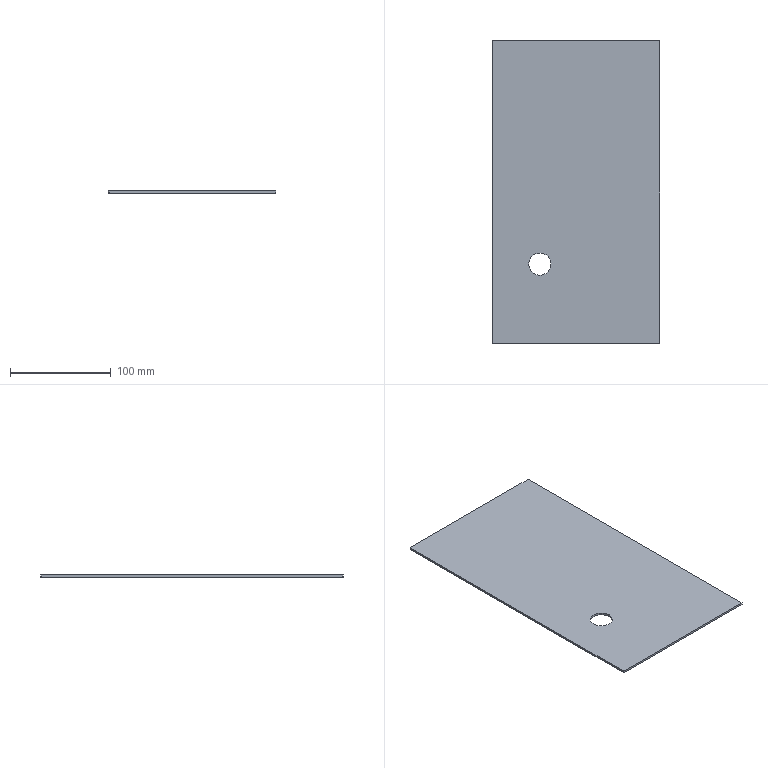Part | STEP file | Oil Filler Tank Closing Plate | 1 solid | 10 faces | box 166.5 x 301 x 2 mm | volume 99472 mm3 | plane 6 | cylinder 4 | commonest cylinder face diameters 1.5 x2 22 x2
STEP:
#1=CARTESIAN_POINT('',(-110.219,-71.7,-2.));
#2=VERTEX_POINT('',#1);
#3=CARTESIAN_POINT('',(-132.219,-71.7,-2.));
#4=VERTEX_POINT('',#3);
#5=CARTESIAN_POINT('',(-121.219,-71.7,-2.));
#6=DIRECTION('',(0.,0.,-1.));
#7=DIRECTION('',(1.,0.,0.));
#8=AXIS2_PLACEMENT_3D('',#5,#6,#7);
#9=CIRCLE('',#8,11.);
#10=EDGE_CURVE('',#2,#4,#9,.T.);
#11=ORIENTED_EDGE('',*,*,#10,.T.);
#12=CARTESIAN_POINT('',(-132.219,-71.7,0.));
#13=VERTEX_POINT('',#12);
#14=CARTESIAN_POINT('',(-132.219,-71.7,-10.));
#15=DIRECTION('',(0.,0.,1.));
#16=VECTOR('',#15,1000.);
#17=LINE('',#14,#16);
#18=EDGE_CURVE('',#4,#13,#17,.T.);
#19=ORIENTED_EDGE('',*,*,#18,.T.);
#20=CARTESIAN_POINT('',(-110.219,-71.7,0.));
#21=VERTEX_POINT('',#20);
#22=CARTESIAN_POINT('',(-121.219,-71.7,0.));
#23=DIRECTION('',(0.,0.,-1.));
#24=DIRECTION('',(1.,0.,0.));
#25=AXIS2_PLACEMENT_3D('',#22,#23,#24);
#26=CIRCLE('',#25,11.);
#27=EDGE_CURVE('',#21,#13,#26,.T.);
#28=ORIENTED_EDGE('',*,*,#27,.F.);
#29=CARTESIAN_POINT('',(-110.219,-71.7,-10.));
#30=DIRECTION('',(0.,0.,1.));
#31=VECTOR('',#30,1000.);
#32=LINE('',#29,#31);
#33=EDGE_CURVE('',#2,#21,#32,.T.);
#34=ORIENTED_EDGE('',*,*,#33,.F.);
#35=EDGE_LOOP('',(#11,#19,#28,#34));
#36=FACE_OUTER_BOUND('',#35,.T.);
#37=CARTESIAN_POINT('',(-121.219,-71.7,-10.));
#38=DIRECTION('',(0.,0.,1.));
#39=DIRECTION('',(1.,0.,0.));
#40=AXIS2_PLACEMENT_3D('',#37,#38,#39);
#41=CYLINDRICAL_SURFACE('',#40,11.);
#42=ADVANCED_FACE('',(#36),#41,.F.);
#43=CARTESIAN_POINT('',(-168.5,-149.75,-2.));
#44=VERTEX_POINT('',#43);
#45=CARTESIAN_POINT('',(-167.75,-150.5,-2.));
#46=VERTEX_POINT('',#45);
#47=CARTESIAN_POINT('',(-167.75,-149.75,-2.));
#48=DIRECTION('',(0.,0.,1.));
#49=DIRECTION('',(1.,0.,0.));
#50=AXIS2_PLACEMENT_3D('',#47,#48,#49);
#51=CIRCLE('',#50,0.75);
#52=EDGE_CURVE('',#44,#46,#51,.T.);
#53=ORIENTED_EDGE('',*,*,#52,.F.);
#54=CARTESIAN_POINT('',(-168.5,149.75,-2.));
#55=VERTEX_POINT('',#54);
#56=CARTESIAN_POINT('',(-168.5,0.,-2.));
#57=DIRECTION('',(0.,-1.,0.));
#58=VECTOR('',#57,1000.);
#59=LINE('',#56,#58);
#60=EDGE_CURVE('',#55,#44,#59,.T.);
#61=ORIENTED_EDGE('',*,*,#60,.F.);
#62=CARTESIAN_POINT('',(-167.75,150.5,-2.));
#63=VERTEX_POINT('',#62);
#64=CARTESIAN_POINT('',(-167.75,149.75,-2.));
#65=DIRECTION('',(0.,0.,1.));
#66=DIRECTION('',(1.,0.,0.));
#67=AXIS2_PLACEMENT_3D('',#64,#65,#66);
#68=CIRCLE('',#67,0.75);
#69=EDGE_CURVE('',#63,#55,#68,.T.);
#70=ORIENTED_EDGE('',*,*,#69,.F.);
#71=CARTESIAN_POINT('',(-2.,150.5,-2.));
#72=VERTEX_POINT('',#71);
#73=CARTESIAN_POINT('',(0.,150.5,-2.));
#74=DIRECTION('',(-1.,0.,0.));
#75=VECTOR('',#74,1000.);
#76=LINE('',#73,#75);
#77=EDGE_CURVE('',#72,#63,#76,.T.);
#78=ORIENTED_EDGE('',*,*,#77,.F.);
#79=CARTESIAN_POINT('',(-2.,-150.5,-2.));
#80=VERTEX_POINT('',#79);
#81=CARTESIAN_POINT('',(-2.,0.,-2.));
#82=DIRECTION('',(0.,1.,0.));
#83=VECTOR('',#82,1000.);
#84=LINE('',#81,#83);
#85=EDGE_CURVE('',#80,#72,#84,.T.);
#86=ORIENTED_EDGE('',*,*,#85,.F.);
#87=CARTESIAN_POINT('',(0.,-150.5,-2.));
#88=DIRECTION('',(1.,0.,0.));
#89=VECTOR('',#88,1000.);
#90=LINE('',#87,#89);
#91=EDGE_CURVE('',#46,#80,#90,.T.);
#92=ORIENTED_EDGE('',*,*,#91,.F.);
#93=EDGE_LOOP('',(#53,#61,#70,#78,#86,#92));
#94=FACE_OUTER_BOUND('',#93,.T.);
#95=ORIENTED_EDGE('',*,*,#10,.F.);
#96=CARTESIAN_POINT('',(-121.219,-71.7,-2.));
#97=DIRECTION('',(0.,0.,-1.));
#98=DIRECTION('',(1.,0.,0.));
#99=AXIS2_PLACEMENT_3D('',#96,#97,#98);
#100=CIRCLE('',#99,11.);
#101=EDGE_CURVE('',#4,#2,#100,.T.);
#102=ORIENTED_EDGE('',*,*,#101,.F.);
#103=EDGE_LOOP('',(#95,#102));
#104=FACE_BOUND('',#103,.T.);
#105=CARTESIAN_POINT('',(0.,0.,-2.));
#106=DIRECTION('',(0.,0.,1.));
#107=DIRECTION('',(1.,0.,0.));
#108=AXIS2_PLACEMENT_3D('',#105,#106,#107);
#109=PLANE('',#108);
#110=ADVANCED_FACE('',(#94,#104),#109,.F.);
#111=ORIENTED_EDGE('',*,*,#91,.T.);
#112=CARTESIAN_POINT('',(-2.,-150.5,0.));
#113=VERTEX_POINT('',#112);
#114=CARTESIAN_POINT('',(-2.,-150.5,-2.));
#115=DIRECTION('',(0.,0.,1.));
#116=VECTOR('',#115,1000.);
#117=LINE('',#114,#116);
#118=EDGE_CURVE('',#80,#113,#117,.T.);
#119=ORIENTED_EDGE('',*,*,#118,.T.);
#120=CARTESIAN_POINT('',(-167.75,-150.5,0.));
#121=VERTEX_POINT('',#120);
#122=CARTESIAN_POINT('',(-168.5,-150.5,0.));
#123=DIRECTION('',(-1.,0.,0.));
#124=VECTOR('',#123,1000.);
#125=LINE('',#122,#124);
#126=EDGE_CURVE('',#113,#121,#125,.T.);
#127=ORIENTED_EDGE('',*,*,#126,.T.);
#128=CARTESIAN_POINT('',(-167.75,-150.5,-2.));
#129=DIRECTION('',(0.,0.,-1.));
#130=VECTOR('',#129,1000.);
#131=LINE('',#128,#130);
#132=EDGE_CURVE('',#121,#46,#131,.T.);
#133=ORIENTED_EDGE('',*,*,#132,.T.);
#134=EDGE_LOOP('',(#111,#119,#127,#133));
#135=FACE_OUTER_BOUND('',#134,.T.);
#136=CARTESIAN_POINT('',(-168.5,-150.5,-2.));
#137=DIRECTION('',(0.,-1.,0.));
#138=DIRECTION('',(0.,0.,-1.));
#139=AXIS2_PLACEMENT_3D('',#136,#137,#138);
#140=PLANE('',#139);
#141=ADVANCED_FACE('',(#135),#140,.T.);
#142=CARTESIAN_POINT('',(-168.5,-149.75,0.));
#143=VERTEX_POINT('',#142);
#144=CARTESIAN_POINT('',(-168.5,149.75,0.));
#145=VERTEX_POINT('',#144);
#146=CARTESIAN_POINT('',(-168.5,150.5,0.));
#147=DIRECTION('',(0.,1.,0.));
#148=VECTOR('',#147,1000.);
#149=LINE('',#146,#148);
#150=EDGE_CURVE('',#143,#145,#149,.T.);
#151=ORIENTED_EDGE('',*,*,#150,.T.);
#152=CARTESIAN_POINT('',(-168.5,149.75,-2.));
#153=DIRECTION('',(0.,0.,-1.));
#154=VECTOR('',#153,1000.);
#155=LINE('',#152,#154);
#156=EDGE_CURVE('',#145,#55,#155,.T.);
#157=ORIENTED_EDGE('',*,*,#156,.T.);
#158=ORIENTED_EDGE('',*,*,#60,.T.);
#159=CARTESIAN_POINT('',(-168.5,-149.75,-2.));
#160=DIRECTION('',(0.,0.,1.));
#161=VECTOR('',#160,1000.);
#162=LINE('',#159,#161);
#163=EDGE_CURVE('',#44,#143,#162,.T.);
#164=ORIENTED_EDGE('',*,*,#163,.T.);
#165=EDGE_LOOP('',(#151,#157,#158,#164));
#166=FACE_OUTER_BOUND('',#165,.T.);
#167=CARTESIAN_POINT('',(-168.5,150.5,-2.));
#168=DIRECTION('',(-1.,0.,0.));
#169=DIRECTION('',(0.,0.,1.));
#170=AXIS2_PLACEMENT_3D('',#167,#168,#169);
#171=PLANE('',#170);
#172=ADVANCED_FACE('',(#166),#171,.T.);
#173=CARTESIAN_POINT('',(-167.75,150.5,0.));
#174=VERTEX_POINT('',#173);
#175=CARTESIAN_POINT('',(-2.,150.5,0.));
#176=VERTEX_POINT('',#175);
#177=CARTESIAN_POINT('',(-168.5,150.5,0.));
#178=DIRECTION('',(1.,0.,0.));
#179=VECTOR('',#178,1000.);
#180=LINE('',#177,#179);
#181=EDGE_CURVE('',#174,#176,#180,.T.);
#182=ORIENTED_EDGE('',*,*,#181,.T.);
#183=CARTESIAN_POINT('',(-2.,150.5,-2.));
#184=DIRECTION('',(0.,0.,-1.));
#185=VECTOR('',#184,1000.);
#186=LINE('',#183,#185);
#187=EDGE_CURVE('',#176,#72,#186,.T.);
#188=ORIENTED_EDGE('',*,*,#187,.T.);
#189=ORIENTED_EDGE('',*,*,#77,.T.);
#190=CARTESIAN_POINT('',(-167.75,150.5,-2.));
#191=DIRECTION('',(0.,0.,1.));
#192=VECTOR('',#191,1000.);
#193=LINE('',#190,#192);
#194=EDGE_CURVE('',#63,#174,#193,.T.);
#195=ORIENTED_EDGE('',*,*,#194,.T.);
#196=EDGE_LOOP('',(#182,#188,#189,#195));
#197=FACE_OUTER_BOUND('',#196,.T.);
#198=CARTESIAN_POINT('',(-168.5,150.5,-2.));
#199=DIRECTION('',(0.,1.,0.));
#200=DIRECTION('',(0.,0.,1.));
#201=AXIS2_PLACEMENT_3D('',#198,#199,#200);
#202=PLANE('',#201);
#203=ADVANCED_FACE('',(#197),#202,.T.);
#204=ORIENTED_EDGE('',*,*,#85,.T.);
#205=ORIENTED_EDGE('',*,*,#187,.F.);
#206=CARTESIAN_POINT('',(-2.,150.5,0.));
#207=DIRECTION('',(0.,-1.,0.));
#208=VECTOR('',#207,1000.);
#209=LINE('',#206,#208);
#210=EDGE_CURVE('',#176,#113,#209,.T.);
#211=ORIENTED_EDGE('',*,*,#210,.T.);
#212=ORIENTED_EDGE('',*,*,#118,.F.);
#213=EDGE_LOOP('',(#204,#205,#211,#212));
#214=FACE_OUTER_BOUND('',#213,.T.);
#215=CARTESIAN_POINT('',(-2.,150.5,-2.));
#216=DIRECTION('',(1.,0.,0.));
#217=DIRECTION('',(0.,0.,-1.));
#218=AXIS2_PLACEMENT_3D('',#215,#216,#217);
#219=PLANE('',#218);
#220=ADVANCED_FACE('',(#214),#219,.T.);
#221=ORIENTED_EDGE('',*,*,#18,.F.);
#222=ORIENTED_EDGE('',*,*,#101,.T.);
#223=ORIENTED_EDGE('',*,*,#33,.T.);
#224=CARTESIAN_POINT('',(-121.219,-71.7,0.));
#225=DIRECTION('',(0.,0.,-1.));
#226=DIRECTION('',(1.,0.,0.));
#227=AXIS2_PLACEMENT_3D('',#224,#225,#226);
#228=CIRCLE('',#227,11.);
#229=EDGE_CURVE('',#13,#21,#228,.T.);
#230=ORIENTED_EDGE('',*,*,#229,.F.);
#231=EDGE_LOOP('',(#221,#222,#223,#230));
#232=FACE_OUTER_BOUND('',#231,.T.);
#233=CARTESIAN_POINT('',(-121.219,-71.7,-10.));
#234=DIRECTION('',(0.,0.,1.));
#235=DIRECTION('',(1.,0.,0.));
#236=AXIS2_PLACEMENT_3D('',#233,#234,#235);
#237=CYLINDRICAL_SURFACE('',#236,11.);
#238=ADVANCED_FACE('',(#232),#237,.F.);
#239=CARTESIAN_POINT('',(-167.75,-149.75,0.));
#240=DIRECTION('',(0.,0.,-1.));
#241=DIRECTION('',(1.,0.,0.));
#242=AXIS2_PLACEMENT_3D('',#239,#240,#241);
#243=CIRCLE('',#242,0.75);
#244=EDGE_CURVE('',#121,#143,#243,.T.);
#245=ORIENTED_EDGE('',*,*,#244,.T.);
#246=ORIENTED_EDGE('',*,*,#163,.F.);
#247=ORIENTED_EDGE('',*,*,#52,.T.);
#248=ORIENTED_EDGE('',*,*,#132,.F.);
#249=EDGE_LOOP('',(#245,#246,#247,#248));
#250=FACE_OUTER_BOUND('',#249,.T.);
#251=CARTESIAN_POINT('',(-167.75,-149.75,-2.));
#252=DIRECTION('',(0.,0.,1.));
#253=DIRECTION('',(1.,0.,0.));
#254=AXIS2_PLACEMENT_3D('',#251,#252,#253);
#255=CYLINDRICAL_SURFACE('',#254,0.75);
#256=ADVANCED_FACE('',(#250),#255,.T.);
#257=ORIENTED_EDGE('',*,*,#181,.F.);
#258=CARTESIAN_POINT('',(-167.75,149.75,0.));
#259=DIRECTION('',(0.,0.,1.));
#260=DIRECTION('',(1.,0.,0.));
#261=AXIS2_PLACEMENT_3D('',#258,#259,#260);
#262=CIRCLE('',#261,0.75);
#263=EDGE_CURVE('',#174,#145,#262,.T.);
#264=ORIENTED_EDGE('',*,*,#263,.T.);
#265=ORIENTED_EDGE('',*,*,#150,.F.);
#266=ORIENTED_EDGE('',*,*,#244,.F.);
#267=ORIENTED_EDGE('',*,*,#126,.F.);
#268=ORIENTED_EDGE('',*,*,#210,.F.);
#269=EDGE_LOOP('',(#257,#264,#265,#266,#267,#268));
#270=FACE_OUTER_BOUND('',#269,.T.);
#271=ORIENTED_EDGE('',*,*,#27,.T.);
#272=ORIENTED_EDGE('',*,*,#229,.T.);
#273=EDGE_LOOP('',(#271,#272));
#274=FACE_BOUND('',#273,.T.);
#275=CARTESIAN_POINT('',(0.,0.,0.));
#276=DIRECTION('',(0.,0.,1.));
#277=DIRECTION('',(1.,0.,0.));
#278=AXIS2_PLACEMENT_3D('',#275,#276,#277);
#279=PLANE('',#278);
#280=ADVANCED_FACE('',(#270,#274),#279,.T.);
#281=ORIENTED_EDGE('',*,*,#263,.F.);
#282=ORIENTED_EDGE('',*,*,#194,.F.);
#283=ORIENTED_EDGE('',*,*,#69,.T.);
#284=ORIENTED_EDGE('',*,*,#156,.F.);
#285=EDGE_LOOP('',(#281,#282,#283,#284));
#286=FACE_OUTER_BOUND('',#285,.T.);
#287=CARTESIAN_POINT('',(-167.75,149.75,-2.));
#288=DIRECTION('',(0.,0.,1.));
#289=DIRECTION('',(1.,0.,0.));
#290=AXIS2_PLACEMENT_3D('',#287,#288,#289);
#291=CYLINDRICAL_SURFACE('',#290,0.75);
#292=ADVANCED_FACE('',(#286),#291,.T.);
#293=CLOSED_SHELL('',(#42,#110,#141,#172,#203,#220,#238,#256,#280,#292));
#294=MANIFOLD_SOLID_BREP('',#293);
#295=CARTESIAN_POINT('',(0.,0.,0.));
#296=DIRECTION('',(0.,0.,1.));
#297=DIRECTION('',(1.,0.,0.));
#298=AXIS2_PLACEMENT_3D('',#295,#296,#297);
#299=(LENGTH_UNIT()NAMED_UNIT(*)SI_UNIT(.MILLI.,.METRE.));
#300=UNCERTAINTY_MEASURE_WITH_UNIT(LENGTH_MEASURE(0.00001),#299,'','');
#301=(NAMED_UNIT(*)PLANE_ANGLE_UNIT()SI_UNIT($,.RADIAN.));
#302=(NAMED_UNIT(*)SI_UNIT($,.STERADIAN.)SOLID_ANGLE_UNIT());
#303=(GEOMETRIC_REPRESENTATION_CONTEXT(3)GLOBAL_UNCERTAINTY_ASSIGNED_CONTEXT((#300))GLOBAL_UNIT_ASSIGNED_CONTEXT((#299,#301,#302))REPRESENTATION_CONTEXT('',''));
#304=ADVANCED_BREP_SHAPE_REPRESENTATION('',(#294,#298),#303);